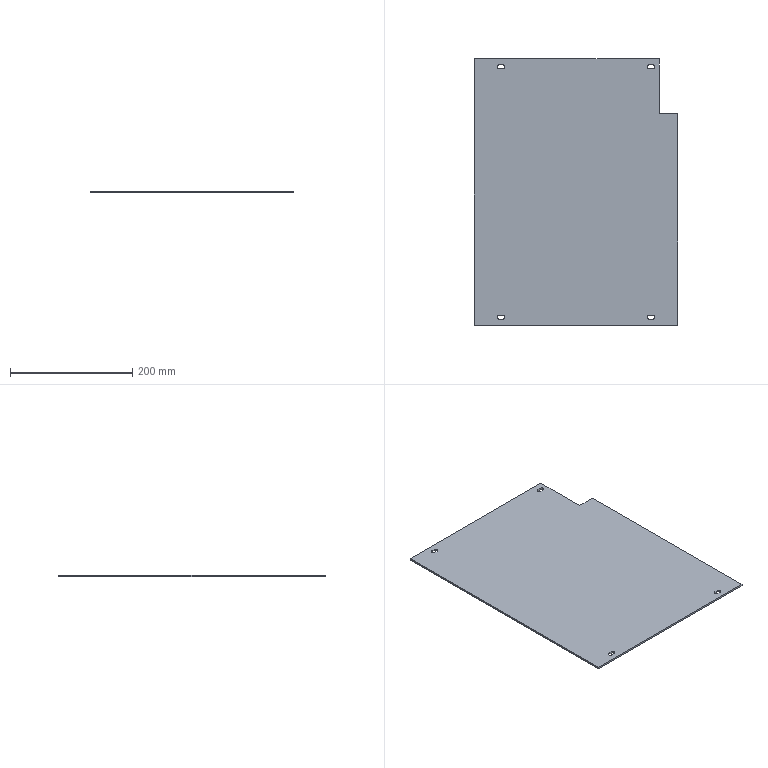Part | SolidWorks | features Cut 2, Extrusion 1 | 1 solid | 28 faces | box 333 x 436 x 3 mm | volume 426578 mm3 | plane 16 | cylinder 12 | commonest cylinder face diameters 6.6 x12
STEP:
#1=CARTESIAN_POINT('',(-116.7,-205.,0.));
#2=VERTEX_POINT('',#1);
#3=CARTESIAN_POINT('',(-120.,-201.7,0.));
#4=VERTEX_POINT('',#3);
#5=CARTESIAN_POINT('',(-120.,-205.,0.));
#6=DIRECTION('',(0.,0.,1.));
#7=DIRECTION('',(1.,0.,0.));
#8=AXIS2_PLACEMENT_3D('',#5,#6,#7);
#9=CIRCLE('',#8,3.3);
#10=EDGE_CURVE('',#2,#4,#9,.T.);
#11=ORIENTED_EDGE('',*,*,#10,.F.);
#12=CARTESIAN_POINT('',(-116.7,-205.,3.));
#13=VERTEX_POINT('',#12);
#14=CARTESIAN_POINT('',(-116.7,-205.,-7.));
#15=DIRECTION('',(0.,0.,1.));
#16=VECTOR('',#15,1000.);
#17=LINE('',#14,#16);
#18=EDGE_CURVE('',#2,#13,#17,.T.);
#19=ORIENTED_EDGE('',*,*,#18,.T.);
#20=CARTESIAN_POINT('',(-120.,-201.7,3.));
#21=VERTEX_POINT('',#20);
#22=CARTESIAN_POINT('',(-120.,-205.,3.));
#23=DIRECTION('',(0.,0.,1.));
#24=DIRECTION('',(1.,0.,0.));
#25=AXIS2_PLACEMENT_3D('',#22,#23,#24);
#26=CIRCLE('',#25,3.3);
#27=EDGE_CURVE('',#13,#21,#26,.T.);
#28=ORIENTED_EDGE('',*,*,#27,.T.);
#29=CARTESIAN_POINT('',(-120.,-201.7,-7.));
#30=DIRECTION('',(0.,0.,1.));
#31=VECTOR('',#30,1000.);
#32=LINE('',#29,#31);
#33=EDGE_CURVE('',#4,#21,#32,.T.);
#34=ORIENTED_EDGE('',*,*,#33,.F.);
#35=EDGE_LOOP('',(#11,#19,#28,#34));
#36=FACE_OUTER_BOUND('',#35,.T.);
#37=CARTESIAN_POINT('',(-120.,-205.,-7.));
#38=DIRECTION('',(0.,0.,1.));
#39=DIRECTION('',(1.,0.,0.));
#40=AXIS2_PLACEMENT_3D('',#37,#38,#39);
#41=CYLINDRICAL_SURFACE('',#40,3.3);
#42=ADVANCED_FACE('',(#36),#41,.F.);
#43=CARTESIAN_POINT('',(129.3,-205.,0.));
#44=VERTEX_POINT('',#43);
#45=CARTESIAN_POINT('',(126.,-201.7,0.));
#46=VERTEX_POINT('',#45);
#47=CARTESIAN_POINT('',(126.,-205.,0.));
#48=DIRECTION('',(0.,0.,1.));
#49=DIRECTION('',(1.,0.,0.));
#50=AXIS2_PLACEMENT_3D('',#47,#48,#49);
#51=CIRCLE('',#50,3.3);
#52=EDGE_CURVE('',#44,#46,#51,.T.);
#53=ORIENTED_EDGE('',*,*,#52,.F.);
#54=CARTESIAN_POINT('',(129.3,-205.,3.));
#55=VERTEX_POINT('',#54);
#56=CARTESIAN_POINT('',(129.3,-205.,-7.));
#57=DIRECTION('',(0.,0.,1.));
#58=VECTOR('',#57,1000.);
#59=LINE('',#56,#58);
#60=EDGE_CURVE('',#44,#55,#59,.T.);
#61=ORIENTED_EDGE('',*,*,#60,.T.);
#62=CARTESIAN_POINT('',(126.,-201.7,3.));
#63=VERTEX_POINT('',#62);
#64=CARTESIAN_POINT('',(126.,-205.,3.));
#65=DIRECTION('',(0.,0.,1.));
#66=DIRECTION('',(1.,0.,0.));
#67=AXIS2_PLACEMENT_3D('',#64,#65,#66);
#68=CIRCLE('',#67,3.3);
#69=EDGE_CURVE('',#55,#63,#68,.T.);
#70=ORIENTED_EDGE('',*,*,#69,.T.);
#71=CARTESIAN_POINT('',(126.,-201.7,-7.));
#72=DIRECTION('',(0.,0.,1.));
#73=VECTOR('',#72,1000.);
#74=LINE('',#71,#73);
#75=EDGE_CURVE('',#46,#63,#74,.T.);
#76=ORIENTED_EDGE('',*,*,#75,.F.);
#77=EDGE_LOOP('',(#53,#61,#70,#76));
#78=FACE_OUTER_BOUND('',#77,.T.);
#79=CARTESIAN_POINT('',(126.,-205.,-7.));
#80=DIRECTION('',(0.,0.,1.));
#81=DIRECTION('',(1.,0.,0.));
#82=AXIS2_PLACEMENT_3D('',#79,#80,#81);
#83=CYLINDRICAL_SURFACE('',#82,3.3);
#84=ADVANCED_FACE('',(#78),#83,.F.);
#85=CARTESIAN_POINT('',(129.3,205.,0.));
#86=VERTEX_POINT('',#85);
#87=CARTESIAN_POINT('',(126.,208.3,0.));
#88=VERTEX_POINT('',#87);
#89=CARTESIAN_POINT('',(126.,205.,0.));
#90=DIRECTION('',(0.,0.,1.));
#91=DIRECTION('',(1.,0.,0.));
#92=AXIS2_PLACEMENT_3D('',#89,#90,#91);
#93=CIRCLE('',#92,3.3);
#94=EDGE_CURVE('',#86,#88,#93,.T.);
#95=ORIENTED_EDGE('',*,*,#94,.F.);
#96=CARTESIAN_POINT('',(129.3,205.,3.));
#97=VERTEX_POINT('',#96);
#98=CARTESIAN_POINT('',(129.3,205.,-7.));
#99=DIRECTION('',(0.,0.,1.));
#100=VECTOR('',#99,1000.);
#101=LINE('',#98,#100);
#102=EDGE_CURVE('',#86,#97,#101,.T.);
#103=ORIENTED_EDGE('',*,*,#102,.T.);
#104=CARTESIAN_POINT('',(126.,208.3,3.));
#105=VERTEX_POINT('',#104);
#106=CARTESIAN_POINT('',(126.,205.,3.));
#107=DIRECTION('',(0.,0.,1.));
#108=DIRECTION('',(1.,0.,0.));
#109=AXIS2_PLACEMENT_3D('',#106,#107,#108);
#110=CIRCLE('',#109,3.3);
#111=EDGE_CURVE('',#97,#105,#110,.T.);
#112=ORIENTED_EDGE('',*,*,#111,.T.);
#113=CARTESIAN_POINT('',(126.,208.3,-7.));
#114=DIRECTION('',(0.,0.,1.));
#115=VECTOR('',#114,1000.);
#116=LINE('',#113,#115);
#117=EDGE_CURVE('',#88,#105,#116,.T.);
#118=ORIENTED_EDGE('',*,*,#117,.F.);
#119=EDGE_LOOP('',(#95,#103,#112,#118));
#120=FACE_OUTER_BOUND('',#119,.T.);
#121=CARTESIAN_POINT('',(126.,205.,-7.));
#122=DIRECTION('',(0.,0.,1.));
#123=DIRECTION('',(1.,0.,0.));
#124=AXIS2_PLACEMENT_3D('',#121,#122,#123);
#125=CYLINDRICAL_SURFACE('',#124,3.3);
#126=ADVANCED_FACE('',(#120),#125,.F.);
#127=CARTESIAN_POINT('',(-116.7,205.,0.));
#128=VERTEX_POINT('',#127);
#129=CARTESIAN_POINT('',(-120.,208.3,0.));
#130=VERTEX_POINT('',#129);
#131=CARTESIAN_POINT('',(-120.,205.,0.));
#132=DIRECTION('',(0.,0.,1.));
#133=DIRECTION('',(1.,0.,0.));
#134=AXIS2_PLACEMENT_3D('',#131,#132,#133);
#135=CIRCLE('',#134,3.3);
#136=EDGE_CURVE('',#128,#130,#135,.T.);
#137=ORIENTED_EDGE('',*,*,#136,.F.);
#138=CARTESIAN_POINT('',(-116.7,205.,3.));
#139=VERTEX_POINT('',#138);
#140=CARTESIAN_POINT('',(-116.7,205.,-7.));
#141=DIRECTION('',(0.,0.,1.));
#142=VECTOR('',#141,1000.);
#143=LINE('',#140,#142);
#144=EDGE_CURVE('',#128,#139,#143,.T.);
#145=ORIENTED_EDGE('',*,*,#144,.T.);
#146=CARTESIAN_POINT('',(-120.,208.3,3.));
#147=VERTEX_POINT('',#146);
#148=CARTESIAN_POINT('',(-120.,205.,3.));
#149=DIRECTION('',(0.,0.,1.));
#150=DIRECTION('',(1.,0.,0.));
#151=AXIS2_PLACEMENT_3D('',#148,#149,#150);
#152=CIRCLE('',#151,3.3);
#153=EDGE_CURVE('',#139,#147,#152,.T.);
#154=ORIENTED_EDGE('',*,*,#153,.T.);
#155=CARTESIAN_POINT('',(-120.,208.3,-7.));
#156=DIRECTION('',(0.,0.,1.));
#157=VECTOR('',#156,1000.);
#158=LINE('',#155,#157);
#159=EDGE_CURVE('',#130,#147,#158,.T.);
#160=ORIENTED_EDGE('',*,*,#159,.F.);
#161=EDGE_LOOP('',(#137,#145,#154,#160));
#162=FACE_OUTER_BOUND('',#161,.T.);
#163=CARTESIAN_POINT('',(-120.,205.,-7.));
#164=DIRECTION('',(0.,0.,1.));
#165=DIRECTION('',(1.,0.,0.));
#166=AXIS2_PLACEMENT_3D('',#163,#164,#165);
#167=CYLINDRICAL_SURFACE('',#166,3.3);
#168=ADVANCED_FACE('',(#162),#167,.F.);
#169=CARTESIAN_POINT('',(-166.5,218.,0.));
#170=VERTEX_POINT('',#169);
#171=CARTESIAN_POINT('',(-166.5,-218.,0.));
#172=VERTEX_POINT('',#171);
#173=CARTESIAN_POINT('',(-166.5,-218.,0.));
#174=DIRECTION('',(0.,-1.,0.));
#175=VECTOR('',#174,1000.);
#176=LINE('',#173,#175);
#177=EDGE_CURVE('',#170,#172,#176,.T.);
#178=ORIENTED_EDGE('',*,*,#177,.T.);
#179=CARTESIAN_POINT('',(-166.5,-218.,3.));
#180=VERTEX_POINT('',#179);
#181=CARTESIAN_POINT('',(-166.5,-218.,3.));
#182=DIRECTION('',(0.,0.,-1.));
#183=VECTOR('',#182,1000.);
#184=LINE('',#181,#183);
#185=EDGE_CURVE('',#180,#172,#184,.T.);
#186=ORIENTED_EDGE('',*,*,#185,.F.);
#187=CARTESIAN_POINT('',(-166.5,218.,3.));
#188=VERTEX_POINT('',#187);
#189=CARTESIAN_POINT('',(-166.5,-218.,3.));
#190=DIRECTION('',(0.,-1.,0.));
#191=VECTOR('',#190,1000.);
#192=LINE('',#189,#191);
#193=EDGE_CURVE('',#188,#180,#192,.T.);
#194=ORIENTED_EDGE('',*,*,#193,.F.);
#195=CARTESIAN_POINT('',(-166.5,218.,3.));
#196=DIRECTION('',(0.,0.,-1.));
#197=VECTOR('',#196,1000.);
#198=LINE('',#195,#197);
#199=EDGE_CURVE('',#188,#170,#198,.T.);
#200=ORIENTED_EDGE('',*,*,#199,.T.);
#201=EDGE_LOOP('',(#178,#186,#194,#200));
#202=FACE_OUTER_BOUND('',#201,.T.);
#203=CARTESIAN_POINT('',(-166.5,-218.,3.));
#204=DIRECTION('',(1.,0.,0.));
#205=DIRECTION('',(0.,0.,-1.));
#206=AXIS2_PLACEMENT_3D('',#203,#204,#205);
#207=PLANE('',#206);
#208=ADVANCED_FACE('',(#202),#207,.F.);
#209=CARTESIAN_POINT('',(166.5,-218.,0.));
#210=VERTEX_POINT('',#209);
#211=CARTESIAN_POINT('',(166.5,-218.,0.));
#212=DIRECTION('',(1.,0.,0.));
#213=VECTOR('',#212,1000.);
#214=LINE('',#211,#213);
#215=EDGE_CURVE('',#172,#210,#214,.T.);
#216=ORIENTED_EDGE('',*,*,#215,.T.);
#217=CARTESIAN_POINT('',(166.5,-218.,3.));
#218=VERTEX_POINT('',#217);
#219=CARTESIAN_POINT('',(166.5,-218.,3.));
#220=DIRECTION('',(0.,0.,-1.));
#221=VECTOR('',#220,1000.);
#222=LINE('',#219,#221);
#223=EDGE_CURVE('',#218,#210,#222,.T.);
#224=ORIENTED_EDGE('',*,*,#223,.F.);
#225=CARTESIAN_POINT('',(166.5,-218.,3.));
#226=DIRECTION('',(1.,0.,0.));
#227=VECTOR('',#226,1000.);
#228=LINE('',#225,#227);
#229=EDGE_CURVE('',#180,#218,#228,.T.);
#230=ORIENTED_EDGE('',*,*,#229,.F.);
#231=ORIENTED_EDGE('',*,*,#185,.T.);
#232=EDGE_LOOP('',(#216,#224,#230,#231));
#233=FACE_OUTER_BOUND('',#232,.T.);
#234=CARTESIAN_POINT('',(166.5,-218.,3.));
#235=DIRECTION('',(0.,1.,0.));
#236=DIRECTION('',(-1.,0.,0.));
#237=AXIS2_PLACEMENT_3D('',#234,#235,#236);
#238=PLANE('',#237);
#239=ADVANCED_FACE('',(#233),#238,.F.);
#240=CARTESIAN_POINT('',(166.5,128.,0.));
#241=VERTEX_POINT('',#240);
#242=CARTESIAN_POINT('',(166.5,-218.,0.));
#243=DIRECTION('',(0.,1.,0.));
#244=VECTOR('',#243,1000.);
#245=LINE('',#242,#244);
#246=EDGE_CURVE('',#210,#241,#245,.T.);
#247=ORIENTED_EDGE('',*,*,#246,.T.);
#248=CARTESIAN_POINT('',(166.5,128.,3.));
#249=VERTEX_POINT('',#248);
#250=CARTESIAN_POINT('',(166.5,128.,10.));
#251=DIRECTION('',(0.,0.,-1.));
#252=VECTOR('',#251,1000.);
#253=LINE('',#250,#252);
#254=EDGE_CURVE('',#249,#241,#253,.T.);
#255=ORIENTED_EDGE('',*,*,#254,.F.);
#256=CARTESIAN_POINT('',(166.5,-218.,3.));
#257=DIRECTION('',(0.,1.,0.));
#258=VECTOR('',#257,1000.);
#259=LINE('',#256,#258);
#260=EDGE_CURVE('',#218,#249,#259,.T.);
#261=ORIENTED_EDGE('',*,*,#260,.F.);
#262=ORIENTED_EDGE('',*,*,#223,.T.);
#263=EDGE_LOOP('',(#247,#255,#261,#262));
#264=FACE_OUTER_BOUND('',#263,.T.);
#265=CARTESIAN_POINT('',(166.5,-218.,3.));
#266=DIRECTION('',(-1.,0.,0.));
#267=DIRECTION('',(0.,0.,1.));
#268=AXIS2_PLACEMENT_3D('',#265,#266,#267);
#269=PLANE('',#268);
#270=ADVANCED_FACE('',(#264),#269,.F.);
#271=CARTESIAN_POINT('',(136.5,218.,3.));
#272=VERTEX_POINT('',#271);
#273=CARTESIAN_POINT('',(166.5,218.,3.));
#274=DIRECTION('',(-1.,0.,0.));
#275=VECTOR('',#274,1000.);
#276=LINE('',#273,#275);
#277=EDGE_CURVE('',#272,#188,#276,.T.);
#278=ORIENTED_EDGE('',*,*,#277,.F.);
#279=CARTESIAN_POINT('',(136.5,218.,0.));
#280=VERTEX_POINT('',#279);
#281=CARTESIAN_POINT('',(136.5,218.,10.));
#282=DIRECTION('',(0.,0.,-1.));
#283=VECTOR('',#282,1000.);
#284=LINE('',#281,#283);
#285=EDGE_CURVE('',#272,#280,#284,.T.);
#286=ORIENTED_EDGE('',*,*,#285,.T.);
#287=CARTESIAN_POINT('',(166.5,218.,0.));
#288=DIRECTION('',(-1.,0.,0.));
#289=VECTOR('',#288,1000.);
#290=LINE('',#287,#289);
#291=EDGE_CURVE('',#280,#170,#290,.T.);
#292=ORIENTED_EDGE('',*,*,#291,.T.);
#293=ORIENTED_EDGE('',*,*,#199,.F.);
#294=EDGE_LOOP('',(#278,#286,#292,#293));
#295=FACE_OUTER_BOUND('',#294,.T.);
#296=CARTESIAN_POINT('',(166.5,218.,3.));
#297=DIRECTION('',(0.,-1.,0.));
#298=DIRECTION('',(1.,0.,0.));
#299=AXIS2_PLACEMENT_3D('',#296,#297,#298);
#300=PLANE('',#299);
#301=ADVANCED_FACE('',(#295),#300,.F.);
#302=CARTESIAN_POINT('',(-120.,-208.3,3.));
#303=VERTEX_POINT('',#302);
#304=CARTESIAN_POINT('',(-120.,-205.,3.));
#305=DIRECTION('',(0.,0.,1.));
#306=DIRECTION('',(1.,0.,0.));
#307=AXIS2_PLACEMENT_3D('',#304,#305,#306);
#308=CIRCLE('',#307,3.3);
#309=EDGE_CURVE('',#303,#13,#308,.T.);
#310=ORIENTED_EDGE('',*,*,#309,.F.);
#311=CARTESIAN_POINT('',(-126.,-208.3,3.));
#312=VERTEX_POINT('',#311);
#313=CARTESIAN_POINT('',(-120.,-208.3,3.));
#314=DIRECTION('',(1.,0.,0.));
#315=VECTOR('',#314,1000.);
#316=LINE('',#313,#315);
#317=EDGE_CURVE('',#312,#303,#316,.T.);
#318=ORIENTED_EDGE('',*,*,#317,.F.);
#319=CARTESIAN_POINT('',(-126.,-201.7,3.));
#320=VERTEX_POINT('',#319);
#321=CARTESIAN_POINT('',(-126.,-205.,3.));
#322=DIRECTION('',(0.,0.,1.));
#323=DIRECTION('',(1.,0.,0.));
#324=AXIS2_PLACEMENT_3D('',#321,#322,#323);
#325=CIRCLE('',#324,3.3);
#326=EDGE_CURVE('',#320,#312,#325,.T.);
#327=ORIENTED_EDGE('',*,*,#326,.F.);
#328=CARTESIAN_POINT('',(-120.,-201.7,3.));
#329=DIRECTION('',(-1.,0.,0.));
#330=VECTOR('',#329,1000.);
#331=LINE('',#328,#330);
#332=EDGE_CURVE('',#21,#320,#331,.T.);
#333=ORIENTED_EDGE('',*,*,#332,.F.);
#334=ORIENTED_EDGE('',*,*,#27,.F.);
#335=EDGE_LOOP('',(#310,#318,#327,#333,#334));
#336=FACE_BOUND('',#335,.T.);
#337=CARTESIAN_POINT('',(120.,-201.7,3.));
#338=VERTEX_POINT('',#337);
#339=CARTESIAN_POINT('',(120.,-208.3,3.));
#340=VERTEX_POINT('',#339);
#341=CARTESIAN_POINT('',(120.,-205.,3.));
#342=DIRECTION('',(0.,0.,1.));
#343=DIRECTION('',(1.,0.,0.));
#344=AXIS2_PLACEMENT_3D('',#341,#342,#343);
#345=CIRCLE('',#344,3.3);
#346=EDGE_CURVE('',#338,#340,#345,.T.);
#347=ORIENTED_EDGE('',*,*,#346,.F.);
#348=CARTESIAN_POINT('',(120.,-201.7,3.));
#349=DIRECTION('',(-1.,0.,0.));
#350=VECTOR('',#349,1000.);
#351=LINE('',#348,#350);
#352=EDGE_CURVE('',#63,#338,#351,.T.);
#353=ORIENTED_EDGE('',*,*,#352,.F.);
#354=ORIENTED_EDGE('',*,*,#69,.F.);
#355=CARTESIAN_POINT('',(126.,-208.3,3.));
#356=VERTEX_POINT('',#355);
#357=CARTESIAN_POINT('',(126.,-205.,3.));
#358=DIRECTION('',(0.,0.,1.));
#359=DIRECTION('',(1.,0.,0.));
#360=AXIS2_PLACEMENT_3D('',#357,#358,#359);
#361=CIRCLE('',#360,3.3);
#362=EDGE_CURVE('',#356,#55,#361,.T.);
#363=ORIENTED_EDGE('',*,*,#362,.F.);
#364=CARTESIAN_POINT('',(120.,-208.3,3.));
#365=DIRECTION('',(1.,0.,0.));
#366=VECTOR('',#365,1000.);
#367=LINE('',#364,#366);
#368=EDGE_CURVE('',#340,#356,#367,.T.);
#369=ORIENTED_EDGE('',*,*,#368,.F.);
#370=EDGE_LOOP('',(#347,#353,#354,#363,#369));
#371=FACE_BOUND('',#370,.T.);
#372=CARTESIAN_POINT('',(120.,208.3,3.));
#373=VERTEX_POINT('',#372);
#374=CARTESIAN_POINT('',(120.,201.7,3.));
#375=VERTEX_POINT('',#374);
#376=CARTESIAN_POINT('',(120.,205.,3.));
#377=DIRECTION('',(0.,0.,1.));
#378=DIRECTION('',(1.,0.,0.));
#379=AXIS2_PLACEMENT_3D('',#376,#377,#378);
#380=CIRCLE('',#379,3.3);
#381=EDGE_CURVE('',#373,#375,#380,.T.);
#382=ORIENTED_EDGE('',*,*,#381,.F.);
#383=CARTESIAN_POINT('',(120.,208.3,3.));
#384=DIRECTION('',(-1.,0.,0.));
#385=VECTOR('',#384,1000.);
#386=LINE('',#383,#385);
#387=EDGE_CURVE('',#105,#373,#386,.T.);
#388=ORIENTED_EDGE('',*,*,#387,.F.);
#389=ORIENTED_EDGE('',*,*,#111,.F.);
#390=CARTESIAN_POINT('',(126.,201.7,3.));
#391=VERTEX_POINT('',#390);
#392=CARTESIAN_POINT('',(126.,205.,3.));
#393=DIRECTION('',(0.,0.,1.));
#394=DIRECTION('',(1.,0.,0.));
#395=AXIS2_PLACEMENT_3D('',#392,#393,#394);
#396=CIRCLE('',#395,3.3);
#397=EDGE_CURVE('',#391,#97,#396,.T.);
#398=ORIENTED_EDGE('',*,*,#397,.F.);
#399=CARTESIAN_POINT('',(120.,201.7,3.));
#400=DIRECTION('',(1.,0.,0.));
#401=VECTOR('',#400,1000.);
#402=LINE('',#399,#401);
#403=EDGE_CURVE('',#375,#391,#402,.T.);
#404=ORIENTED_EDGE('',*,*,#403,.F.);
#405=EDGE_LOOP('',(#382,#388,#389,#398,#404));
#406=FACE_BOUND('',#405,.T.);
#407=CARTESIAN_POINT('',(-120.,201.7,3.));
#408=VERTEX_POINT('',#407);
#409=CARTESIAN_POINT('',(-120.,205.,3.));
#410=DIRECTION('',(0.,0.,1.));
#411=DIRECTION('',(1.,0.,0.));
#412=AXIS2_PLACEMENT_3D('',#409,#410,#411);
#413=CIRCLE('',#412,3.3);
#414=EDGE_CURVE('',#408,#139,#413,.T.);
#415=ORIENTED_EDGE('',*,*,#414,.F.);
#416=CARTESIAN_POINT('',(-126.,201.7,3.));
#417=VERTEX_POINT('',#416);
#418=CARTESIAN_POINT('',(-120.,201.7,3.));
#419=DIRECTION('',(1.,0.,0.));
#420=VECTOR('',#419,1000.);
#421=LINE('',#418,#420);
#422=EDGE_CURVE('',#417,#408,#421,.T.);
#423=ORIENTED_EDGE('',*,*,#422,.F.);
#424=CARTESIAN_POINT('',(-126.,208.3,3.));
#425=VERTEX_POINT('',#424);
#426=CARTESIAN_POINT('',(-126.,205.,3.));
#427=DIRECTION('',(0.,0.,1.));
#428=DIRECTION('',(1.,0.,0.));
#429=AXIS2_PLACEMENT_3D('',#426,#427,#428);
#430=CIRCLE('',#429,3.3);
#431=EDGE_CURVE('',#425,#417,#430,.T.);
#432=ORIENTED_EDGE('',*,*,#431,.F.);
#433=CARTESIAN_POINT('',(-120.,208.3,3.));
#434=DIRECTION('',(-1.,0.,0.));
#435=VECTOR('',#434,1000.);
#436=LINE('',#433,#435);
#437=EDGE_CURVE('',#147,#425,#436,.T.);
#438=ORIENTED_EDGE('',*,*,#437,.F.);
#439=ORIENTED_EDGE('',*,*,#153,.F.);
#440=EDGE_LOOP('',(#415,#423,#432,#438,#439));
#441=FACE_BOUND('',#440,.T.);
#442=CARTESIAN_POINT('',(136.5,128.,3.));
#443=VERTEX_POINT('',#442);
#444=CARTESIAN_POINT('',(136.5,0.,3.));
#445=DIRECTION('',(0.,-1.,0.));
#446=VECTOR('',#445,1000.);
#447=LINE('',#444,#446);
#448=EDGE_CURVE('',#272,#443,#447,.T.);
#449=ORIENTED_EDGE('',*,*,#448,.F.);
#450=ORIENTED_EDGE('',*,*,#277,.T.);
#451=ORIENTED_EDGE('',*,*,#193,.T.);
#452=ORIENTED_EDGE('',*,*,#229,.T.);
#453=ORIENTED_EDGE('',*,*,#260,.T.);
#454=CARTESIAN_POINT('',(0.,128.,3.));
#455=DIRECTION('',(1.,0.,0.));
#456=VECTOR('',#455,1000.);
#457=LINE('',#454,#456);
#458=EDGE_CURVE('',#443,#249,#457,.T.);
#459=ORIENTED_EDGE('',*,*,#458,.F.);
#460=EDGE_LOOP('',(#449,#450,#451,#452,#453,#459));
#461=FACE_OUTER_BOUND('',#460,.T.);
#462=CARTESIAN_POINT('',(0.,0.,3.));
#463=DIRECTION('',(0.,0.,1.));
#464=DIRECTION('',(1.,0.,0.));
#465=AXIS2_PLACEMENT_3D('',#462,#463,#464);
#466=PLANE('',#465);
#467=ADVANCED_FACE('',(#336,#371,#406,#441,#461),#466,.T.);
#468=CARTESIAN_POINT('',(-126.,-208.3,0.));
#469=VERTEX_POINT('',#468);
#470=CARTESIAN_POINT('',(-120.,-208.3,0.));
#471=VERTEX_POINT('',#470);
#472=CARTESIAN_POINT('',(0.,-208.3,0.));
#473=DIRECTION('',(1.,0.,0.));
#474=VECTOR('',#473,1000.);
#475=LINE('',#472,#474);
#476=EDGE_CURVE('',#469,#471,#475,.T.);
#477=ORIENTED_EDGE('',*,*,#476,.T.);
#478=CARTESIAN_POINT('',(-120.,-205.,0.));
#479=DIRECTION('',(0.,0.,1.));
#480=DIRECTION('',(1.,0.,0.));
#481=AXIS2_PLACEMENT_3D('',#478,#479,#480);
#482=CIRCLE('',#481,3.3);
#483=EDGE_CURVE('',#471,#2,#482,.T.);
#484=ORIENTED_EDGE('',*,*,#483,.T.);
#485=ORIENTED_EDGE('',*,*,#10,.T.);
#486=CARTESIAN_POINT('',(-126.,-201.7,0.));
#487=VERTEX_POINT('',#486);
#488=CARTESIAN_POINT('',(0.,-201.7,0.));
#489=DIRECTION('',(-1.,0.,0.));
#490=VECTOR('',#489,1000.);
#491=LINE('',#488,#490);
#492=EDGE_CURVE('',#4,#487,#491,.T.);
#493=ORIENTED_EDGE('',*,*,#492,.T.);
#494=CARTESIAN_POINT('',(-126.,-205.,0.));
#495=DIRECTION('',(0.,0.,1.));
#496=DIRECTION('',(1.,0.,0.));
#497=AXIS2_PLACEMENT_3D('',#494,#495,#496);
#498=CIRCLE('',#497,3.3);
#499=EDGE_CURVE('',#487,#469,#498,.T.);
#500=ORIENTED_EDGE('',*,*,#499,.T.);
#501=EDGE_LOOP('',(#477,#484,#485,#493,#500));
#502=FACE_BOUND('',#501,.T.);
#503=CARTESIAN_POINT('',(120.,-201.7,0.));
#504=VERTEX_POINT('',#503);
#505=CARTESIAN_POINT('',(0.,-201.7,0.));
#506=DIRECTION('',(-1.,0.,0.));
#507=VECTOR('',#506,1000.);
#508=LINE('',#505,#507);
#509=EDGE_CURVE('',#46,#504,#508,.T.);
#510=ORIENTED_EDGE('',*,*,#509,.T.);
#511=CARTESIAN_POINT('',(120.,-208.3,0.));
#512=VERTEX_POINT('',#511);
#513=CARTESIAN_POINT('',(120.,-205.,0.));
#514=DIRECTION('',(0.,0.,1.));
#515=DIRECTION('',(1.,0.,0.));
#516=AXIS2_PLACEMENT_3D('',#513,#514,#515);
#517=CIRCLE('',#516,3.3);
#518=EDGE_CURVE('',#504,#512,#517,.T.);
#519=ORIENTED_EDGE('',*,*,#518,.T.);
#520=CARTESIAN_POINT('',(126.,-208.3,0.));
#521=VERTEX_POINT('',#520);
#522=CARTESIAN_POINT('',(0.,-208.3,0.));
#523=DIRECTION('',(1.,0.,0.));
#524=VECTOR('',#523,1000.);
#525=LINE('',#522,#524);
#526=EDGE_CURVE('',#512,#521,#525,.T.);
#527=ORIENTED_EDGE('',*,*,#526,.T.);
#528=CARTESIAN_POINT('',(126.,-205.,0.));
#529=DIRECTION('',(0.,0.,1.));
#530=DIRECTION('',(1.,0.,0.));
#531=AXIS2_PLACEMENT_3D('',#528,#529,#530);
#532=CIRCLE('',#531,3.3);
#533=EDGE_CURVE('',#521,#44,#532,.T.);
#534=ORIENTED_EDGE('',*,*,#533,.T.);
#535=ORIENTED_EDGE('',*,*,#52,.T.);
#536=EDGE_LOOP('',(#510,#519,#527,#534,#535));
#537=FACE_BOUND('',#536,.T.);
#538=CARTESIAN_POINT('',(120.,208.3,0.));
#539=VERTEX_POINT('',#538);
#540=CARTESIAN_POINT('',(0.,208.3,0.));
#541=DIRECTION('',(-1.,0.,0.));
#542=VECTOR('',#541,1000.);
#543=LINE('',#540,#542);
#544=EDGE_CURVE('',#88,#539,#543,.T.);
#545=ORIENTED_EDGE('',*,*,#544,.T.);
#546=CARTESIAN_POINT('',(120.,201.7,0.));
#547=VERTEX_POINT('',#546);
#548=CARTESIAN_POINT('',(120.,205.,0.));
#549=DIRECTION('',(0.,0.,1.));
#550=DIRECTION('',(1.,0.,0.));
#551=AXIS2_PLACEMENT_3D('',#548,#549,#550);
#552=CIRCLE('',#551,3.3);
#553=EDGE_CURVE('',#539,#547,#552,.T.);
#554=ORIENTED_EDGE('',*,*,#553,.T.);
#555=CARTESIAN_POINT('',(126.,201.7,0.));
#556=VERTEX_POINT('',#555);
#557=CARTESIAN_POINT('',(0.,201.7,0.));
#558=DIRECTION('',(1.,0.,0.));
#559=VECTOR('',#558,1000.);
#560=LINE('',#557,#559);
#561=EDGE_CURVE('',#547,#556,#560,.T.);
#562=ORIENTED_EDGE('',*,*,#561,.T.);
#563=CARTESIAN_POINT('',(126.,205.,0.));
#564=DIRECTION('',(0.,0.,1.));
#565=DIRECTION('',(1.,0.,0.));
#566=AXIS2_PLACEMENT_3D('',#563,#564,#565);
#567=CIRCLE('',#566,3.3);
#568=EDGE_CURVE('',#556,#86,#567,.T.);
#569=ORIENTED_EDGE('',*,*,#568,.T.);
#570=ORIENTED_EDGE('',*,*,#94,.T.);
#571=EDGE_LOOP('',(#545,#554,#562,#569,#570));
#572=FACE_BOUND('',#571,.T.);
#573=CARTESIAN_POINT('',(-126.,201.7,0.));
#574=VERTEX_POINT('',#573);
#575=CARTESIAN_POINT('',(-120.,201.7,0.));
#576=VERTEX_POINT('',#575);
#577=CARTESIAN_POINT('',(0.,201.7,0.));
#578=DIRECTION('',(1.,0.,0.));
#579=VECTOR('',#578,1000.);
#580=LINE('',#577,#579);
#581=EDGE_CURVE('',#574,#576,#580,.T.);
#582=ORIENTED_EDGE('',*,*,#581,.T.);
#583=CARTESIAN_POINT('',(-120.,205.,0.));
#584=DIRECTION('',(0.,0.,1.));
#585=DIRECTION('',(1.,0.,0.));
#586=AXIS2_PLACEMENT_3D('',#583,#584,#585);
#587=CIRCLE('',#586,3.3);
#588=EDGE_CURVE('',#576,#128,#587,.T.);
#589=ORIENTED_EDGE('',*,*,#588,.T.);
#590=ORIENTED_EDGE('',*,*,#136,.T.);
#591=CARTESIAN_POINT('',(-126.,208.3,0.));
#592=VERTEX_POINT('',#591);
#593=CARTESIAN_POINT('',(0.,208.3,0.));
#594=DIRECTION('',(-1.,0.,0.));
#595=VECTOR('',#594,1000.);
#596=LINE('',#593,#595);
#597=EDGE_CURVE('',#130,#592,#596,.T.);
#598=ORIENTED_EDGE('',*,*,#597,.T.);
#599=CARTESIAN_POINT('',(-126.,205.,0.));
#600=DIRECTION('',(0.,0.,1.));
#601=DIRECTION('',(1.,0.,0.));
#602=AXIS2_PLACEMENT_3D('',#599,#600,#601);
#603=CIRCLE('',#602,3.3);
#604=EDGE_CURVE('',#592,#574,#603,.T.);
#605=ORIENTED_EDGE('',*,*,#604,.T.);
#606=EDGE_LOOP('',(#582,#589,#590,#598,#605));
#607=FACE_BOUND('',#606,.T.);
#608=ORIENTED_EDGE('',*,*,#291,.F.);
#609=CARTESIAN_POINT('',(136.5,128.,0.));
#610=VERTEX_POINT('',#609);
#611=CARTESIAN_POINT('',(136.5,128.,0.));
#612=DIRECTION('',(0.,1.,0.));
#613=VECTOR('',#612,1000.);
#614=LINE('',#611,#613);
#615=EDGE_CURVE('',#610,#280,#614,.T.);
#616=ORIENTED_EDGE('',*,*,#615,.F.);
#617=CARTESIAN_POINT('',(136.5,128.,0.));
#618=DIRECTION('',(-1.,0.,0.));
#619=VECTOR('',#618,1000.);
#620=LINE('',#617,#619);
#621=EDGE_CURVE('',#241,#610,#620,.T.);
#622=ORIENTED_EDGE('',*,*,#621,.F.);
#623=ORIENTED_EDGE('',*,*,#246,.F.);
#624=ORIENTED_EDGE('',*,*,#215,.F.);
#625=ORIENTED_EDGE('',*,*,#177,.F.);
#626=EDGE_LOOP('',(#608,#616,#622,#623,#624,#625));
#627=FACE_OUTER_BOUND('',#626,.T.);
#628=CARTESIAN_POINT('',(0.,0.,0.));
#629=DIRECTION('',(0.,0.,1.));
#630=DIRECTION('',(1.,0.,0.));
#631=AXIS2_PLACEMENT_3D('',#628,#629,#630);
#632=PLANE('',#631);
#633=ADVANCED_FACE('',(#502,#537,#572,#607,#627),#632,.F.);
#634=ORIENTED_EDGE('',*,*,#448,.T.);
#635=CARTESIAN_POINT('',(136.5,128.,10.));
#636=DIRECTION('',(0.,0.,-1.));
#637=VECTOR('',#636,1000.);
#638=LINE('',#635,#637);
#639=EDGE_CURVE('',#443,#610,#638,.T.);
#640=ORIENTED_EDGE('',*,*,#639,.T.);
#641=ORIENTED_EDGE('',*,*,#615,.T.);
#642=ORIENTED_EDGE('',*,*,#285,.F.);
#643=EDGE_LOOP('',(#634,#640,#641,#642));
#644=FACE_OUTER_BOUND('',#643,.T.);
#645=CARTESIAN_POINT('',(136.5,128.,10.));
#646=DIRECTION('',(-1.,0.,0.));
#647=DIRECTION('',(0.,0.,1.));
#648=AXIS2_PLACEMENT_3D('',#645,#646,#647);
#649=PLANE('',#648);
#650=ADVANCED_FACE('',(#644),#649,.F.);
#651=ORIENTED_EDGE('',*,*,#458,.T.);
#652=ORIENTED_EDGE('',*,*,#254,.T.);
#653=ORIENTED_EDGE('',*,*,#621,.T.);
#654=ORIENTED_EDGE('',*,*,#639,.F.);
#655=EDGE_LOOP('',(#651,#652,#653,#654));
#656=FACE_OUTER_BOUND('',#655,.T.);
#657=CARTESIAN_POINT('',(136.5,128.,10.));
#658=DIRECTION('',(0.,-1.,0.));
#659=DIRECTION('',(1.,0.,0.));
#660=AXIS2_PLACEMENT_3D('',#657,#658,#659);
#661=PLANE('',#660);
#662=ADVANCED_FACE('',(#656),#661,.F.);
#663=ORIENTED_EDGE('',*,*,#144,.F.);
#664=ORIENTED_EDGE('',*,*,#588,.F.);
#665=CARTESIAN_POINT('',(-120.,201.7,-7.));
#666=DIRECTION('',(0.,0.,1.));
#667=VECTOR('',#666,1000.);
#668=LINE('',#665,#667);
#669=EDGE_CURVE('',#576,#408,#668,.T.);
#670=ORIENTED_EDGE('',*,*,#669,.T.);
#671=ORIENTED_EDGE('',*,*,#414,.T.);
#672=EDGE_LOOP('',(#663,#664,#670,#671));
#673=FACE_OUTER_BOUND('',#672,.T.);
#674=CARTESIAN_POINT('',(-120.,205.,-7.));
#675=DIRECTION('',(0.,0.,1.));
#676=DIRECTION('',(1.,0.,0.));
#677=AXIS2_PLACEMENT_3D('',#674,#675,#676);
#678=CYLINDRICAL_SURFACE('',#677,3.3);
#679=ADVANCED_FACE('',(#673),#678,.F.);
#680=CARTESIAN_POINT('',(-126.,201.7,-7.));
#681=DIRECTION('',(0.,0.,1.));
#682=VECTOR('',#681,1000.);
#683=LINE('',#680,#682);
#684=EDGE_CURVE('',#574,#417,#683,.T.);
#685=ORIENTED_EDGE('',*,*,#684,.T.);
#686=ORIENTED_EDGE('',*,*,#422,.T.);
#687=ORIENTED_EDGE('',*,*,#669,.F.);
#688=ORIENTED_EDGE('',*,*,#581,.F.);
#689=EDGE_LOOP('',(#685,#686,#687,#688));
#690=FACE_OUTER_BOUND('',#689,.T.);
#691=CARTESIAN_POINT('',(-120.,201.7,-7.));
#692=DIRECTION('',(0.,-1.,0.));
#693=DIRECTION('',(1.,0.,0.));
#694=AXIS2_PLACEMENT_3D('',#691,#692,#693);
#695=PLANE('',#694);
#696=ADVANCED_FACE('',(#690),#695,.F.);
#697=CARTESIAN_POINT('',(-126.,208.3,-7.));
#698=DIRECTION('',(0.,0.,1.));
#699=VECTOR('',#698,1000.);
#700=LINE('',#697,#699);
#701=EDGE_CURVE('',#592,#425,#700,.T.);
#702=ORIENTED_EDGE('',*,*,#701,.T.);
#703=ORIENTED_EDGE('',*,*,#431,.T.);
#704=ORIENTED_EDGE('',*,*,#684,.F.);
#705=ORIENTED_EDGE('',*,*,#604,.F.);
#706=EDGE_LOOP('',(#702,#703,#704,#705));
#707=FACE_OUTER_BOUND('',#706,.T.);
#708=CARTESIAN_POINT('',(-126.,205.,-7.));
#709=DIRECTION('',(0.,0.,1.));
#710=DIRECTION('',(1.,0.,0.));
#711=AXIS2_PLACEMENT_3D('',#708,#709,#710);
#712=CYLINDRICAL_SURFACE('',#711,3.3);
#713=ADVANCED_FACE('',(#707),#712,.F.);
#714=ORIENTED_EDGE('',*,*,#159,.T.);
#715=ORIENTED_EDGE('',*,*,#437,.T.);
#716=ORIENTED_EDGE('',*,*,#701,.F.);
#717=ORIENTED_EDGE('',*,*,#597,.F.);
#718=EDGE_LOOP('',(#714,#715,#716,#717));
#719=FACE_OUTER_BOUND('',#718,.T.);
#720=CARTESIAN_POINT('',(-120.,208.3,-7.));
#721=DIRECTION('',(0.,1.,0.));
#722=DIRECTION('',(-1.,0.,0.));
#723=AXIS2_PLACEMENT_3D('',#720,#721,#722);
#724=PLANE('',#723);
#725=ADVANCED_FACE('',(#719),#724,.F.);
#726=CARTESIAN_POINT('',(120.,208.3,-7.));
#727=DIRECTION('',(0.,0.,1.));
#728=VECTOR('',#727,1000.);
#729=LINE('',#726,#728);
#730=EDGE_CURVE('',#539,#373,#729,.T.);
#731=ORIENTED_EDGE('',*,*,#730,.T.);
#732=ORIENTED_EDGE('',*,*,#381,.T.);
#733=CARTESIAN_POINT('',(120.,201.7,-7.));
#734=DIRECTION('',(0.,0.,1.));
#735=VECTOR('',#734,1000.);
#736=LINE('',#733,#735);
#737=EDGE_CURVE('',#547,#375,#736,.T.);
#738=ORIENTED_EDGE('',*,*,#737,.F.);
#739=ORIENTED_EDGE('',*,*,#553,.F.);
#740=EDGE_LOOP('',(#731,#732,#738,#739));
#741=FACE_OUTER_BOUND('',#740,.T.);
#742=CARTESIAN_POINT('',(120.,205.,-7.));
#743=DIRECTION('',(0.,0.,1.));
#744=DIRECTION('',(1.,0.,0.));
#745=AXIS2_PLACEMENT_3D('',#742,#743,#744);
#746=CYLINDRICAL_SURFACE('',#745,3.3);
#747=ADVANCED_FACE('',(#741),#746,.F.);
#748=ORIENTED_EDGE('',*,*,#117,.T.);
#749=ORIENTED_EDGE('',*,*,#387,.T.);
#750=ORIENTED_EDGE('',*,*,#730,.F.);
#751=ORIENTED_EDGE('',*,*,#544,.F.);
#752=EDGE_LOOP('',(#748,#749,#750,#751));
#753=FACE_OUTER_BOUND('',#752,.T.);
#754=CARTESIAN_POINT('',(120.,208.3,-7.));
#755=DIRECTION('',(0.,1.,0.));
#756=DIRECTION('',(0.,0.,1.));
#757=AXIS2_PLACEMENT_3D('',#754,#755,#756);
#758=PLANE('',#757);
#759=ADVANCED_FACE('',(#753),#758,.F.);
#760=ORIENTED_EDGE('',*,*,#102,.F.);
#761=ORIENTED_EDGE('',*,*,#568,.F.);
#762=CARTESIAN_POINT('',(126.,201.7,-7.));
#763=DIRECTION('',(0.,0.,1.));
#764=VECTOR('',#763,1000.);
#765=LINE('',#762,#764);
#766=EDGE_CURVE('',#556,#391,#765,.T.);
#767=ORIENTED_EDGE('',*,*,#766,.T.);
#768=ORIENTED_EDGE('',*,*,#397,.T.);
#769=EDGE_LOOP('',(#760,#761,#767,#768));
#770=FACE_OUTER_BOUND('',#769,.T.);
#771=CARTESIAN_POINT('',(126.,205.,-7.));
#772=DIRECTION('',(0.,0.,1.));
#773=DIRECTION('',(1.,0.,0.));
#774=AXIS2_PLACEMENT_3D('',#771,#772,#773);
#775=CYLINDRICAL_SURFACE('',#774,3.3);
#776=ADVANCED_FACE('',(#770),#775,.F.);
#777=ORIENTED_EDGE('',*,*,#737,.T.);
#778=ORIENTED_EDGE('',*,*,#403,.T.);
#779=ORIENTED_EDGE('',*,*,#766,.F.);
#780=ORIENTED_EDGE('',*,*,#561,.F.);
#781=EDGE_LOOP('',(#777,#778,#779,#780));
#782=FACE_OUTER_BOUND('',#781,.T.);
#783=CARTESIAN_POINT('',(120.,201.7,-7.));
#784=DIRECTION('',(0.,-1.,0.));
#785=DIRECTION('',(0.,0.,-1.));
#786=AXIS2_PLACEMENT_3D('',#783,#784,#785);
#787=PLANE('',#786);
#788=ADVANCED_FACE('',(#782),#787,.F.);
#789=CARTESIAN_POINT('',(120.,-201.7,-7.));
#790=DIRECTION('',(0.,0.,1.));
#791=VECTOR('',#790,1000.);
#792=LINE('',#789,#791);
#793=EDGE_CURVE('',#504,#338,#792,.T.);
#794=ORIENTED_EDGE('',*,*,#793,.T.);
#795=ORIENTED_EDGE('',*,*,#346,.T.);
#796=CARTESIAN_POINT('',(120.,-208.3,-7.));
#797=DIRECTION('',(0.,0.,1.));
#798=VECTOR('',#797,1000.);
#799=LINE('',#796,#798);
#800=EDGE_CURVE('',#512,#340,#799,.T.);
#801=ORIENTED_EDGE('',*,*,#800,.F.);
#802=ORIENTED_EDGE('',*,*,#518,.F.);
#803=EDGE_LOOP('',(#794,#795,#801,#802));
#804=FACE_OUTER_BOUND('',#803,.T.);
#805=CARTESIAN_POINT('',(120.,-205.,-7.));
#806=DIRECTION('',(0.,0.,1.));
#807=DIRECTION('',(1.,0.,0.));
#808=AXIS2_PLACEMENT_3D('',#805,#806,#807);
#809=CYLINDRICAL_SURFACE('',#808,3.3);
#810=ADVANCED_FACE('',(#804),#809,.F.);
#811=ORIENTED_EDGE('',*,*,#75,.T.);
#812=ORIENTED_EDGE('',*,*,#352,.T.);
#813=ORIENTED_EDGE('',*,*,#793,.F.);
#814=ORIENTED_EDGE('',*,*,#509,.F.);
#815=EDGE_LOOP('',(#811,#812,#813,#814));
#816=FACE_OUTER_BOUND('',#815,.T.);
#817=CARTESIAN_POINT('',(120.,-201.7,-7.));
#818=DIRECTION('',(0.,1.,0.));
#819=DIRECTION('',(-1.,0.,0.));
#820=AXIS2_PLACEMENT_3D('',#817,#818,#819);
#821=PLANE('',#820);
#822=ADVANCED_FACE('',(#816),#821,.F.);
#823=ORIENTED_EDGE('',*,*,#60,.F.);
#824=ORIENTED_EDGE('',*,*,#533,.F.);
#825=CARTESIAN_POINT('',(126.,-208.3,-7.));
#826=DIRECTION('',(0.,0.,1.));
#827=VECTOR('',#826,1000.);
#828=LINE('',#825,#827);
#829=EDGE_CURVE('',#521,#356,#828,.T.);
#830=ORIENTED_EDGE('',*,*,#829,.T.);
#831=ORIENTED_EDGE('',*,*,#362,.T.);
#832=EDGE_LOOP('',(#823,#824,#830,#831));
#833=FACE_OUTER_BOUND('',#832,.T.);
#834=CARTESIAN_POINT('',(126.,-205.,-7.));
#835=DIRECTION('',(0.,0.,1.));
#836=DIRECTION('',(1.,0.,0.));
#837=AXIS2_PLACEMENT_3D('',#834,#835,#836);
#838=CYLINDRICAL_SURFACE('',#837,3.3);
#839=ADVANCED_FACE('',(#833),#838,.F.);
#840=ORIENTED_EDGE('',*,*,#800,.T.);
#841=ORIENTED_EDGE('',*,*,#368,.T.);
#842=ORIENTED_EDGE('',*,*,#829,.F.);
#843=ORIENTED_EDGE('',*,*,#526,.F.);
#844=EDGE_LOOP('',(#840,#841,#842,#843));
#845=FACE_OUTER_BOUND('',#844,.T.);
#846=CARTESIAN_POINT('',(120.,-208.3,-7.));
#847=DIRECTION('',(0.,-1.,0.));
#848=DIRECTION('',(1.,0.,0.));
#849=AXIS2_PLACEMENT_3D('',#846,#847,#848);
#850=PLANE('',#849);
#851=ADVANCED_FACE('',(#845),#850,.F.);
#852=ORIENTED_EDGE('',*,*,#18,.F.);
#853=ORIENTED_EDGE('',*,*,#483,.F.);
#854=CARTESIAN_POINT('',(-120.,-208.3,-7.));
#855=DIRECTION('',(0.,0.,1.));
#856=VECTOR('',#855,1000.);
#857=LINE('',#854,#856);
#858=EDGE_CURVE('',#471,#303,#857,.T.);
#859=ORIENTED_EDGE('',*,*,#858,.T.);
#860=ORIENTED_EDGE('',*,*,#309,.T.);
#861=EDGE_LOOP('',(#852,#853,#859,#860));
#862=FACE_OUTER_BOUND('',#861,.T.);
#863=CARTESIAN_POINT('',(-120.,-205.,-7.));
#864=DIRECTION('',(0.,0.,1.));
#865=DIRECTION('',(1.,0.,0.));
#866=AXIS2_PLACEMENT_3D('',#863,#864,#865);
#867=CYLINDRICAL_SURFACE('',#866,3.3);
#868=ADVANCED_FACE('',(#862),#867,.F.);
#869=CARTESIAN_POINT('',(-126.,-208.3,-7.));
#870=DIRECTION('',(0.,0.,1.));
#871=VECTOR('',#870,1000.);
#872=LINE('',#869,#871);
#873=EDGE_CURVE('',#469,#312,#872,.T.);
#874=ORIENTED_EDGE('',*,*,#873,.T.);
#875=ORIENTED_EDGE('',*,*,#317,.T.);
#876=ORIENTED_EDGE('',*,*,#858,.F.);
#877=ORIENTED_EDGE('',*,*,#476,.F.);
#878=EDGE_LOOP('',(#874,#875,#876,#877));
#879=FACE_OUTER_BOUND('',#878,.T.);
#880=CARTESIAN_POINT('',(-120.,-208.3,-7.));
#881=DIRECTION('',(0.,-1.,0.));
#882=DIRECTION('',(1.,0.,0.));
#883=AXIS2_PLACEMENT_3D('',#880,#881,#882);
#884=PLANE('',#883);
#885=ADVANCED_FACE('',(#879),#884,.F.);
#886=CARTESIAN_POINT('',(-126.,-201.7,-7.));
#887=DIRECTION('',(0.,0.,1.));
#888=VECTOR('',#887,1000.);
#889=LINE('',#886,#888);
#890=EDGE_CURVE('',#487,#320,#889,.T.);
#891=ORIENTED_EDGE('',*,*,#890,.T.);
#892=ORIENTED_EDGE('',*,*,#326,.T.);
#893=ORIENTED_EDGE('',*,*,#873,.F.);
#894=ORIENTED_EDGE('',*,*,#499,.F.);
#895=EDGE_LOOP('',(#891,#892,#893,#894));
#896=FACE_OUTER_BOUND('',#895,.T.);
#897=CARTESIAN_POINT('',(-126.,-205.,-7.));
#898=DIRECTION('',(0.,0.,1.));
#899=DIRECTION('',(1.,0.,0.));
#900=AXIS2_PLACEMENT_3D('',#897,#898,#899);
#901=CYLINDRICAL_SURFACE('',#900,3.3);
#902=ADVANCED_FACE('',(#896),#901,.F.);
#903=ORIENTED_EDGE('',*,*,#33,.T.);
#904=ORIENTED_EDGE('',*,*,#332,.T.);
#905=ORIENTED_EDGE('',*,*,#890,.F.);
#906=ORIENTED_EDGE('',*,*,#492,.F.);
#907=EDGE_LOOP('',(#903,#904,#905,#906));
#908=FACE_OUTER_BOUND('',#907,.T.);
#909=CARTESIAN_POINT('',(-120.,-201.7,-7.));
#910=DIRECTION('',(0.,1.,0.));
#911=DIRECTION('',(-1.,0.,0.));
#912=AXIS2_PLACEMENT_3D('',#909,#910,#911);
#913=PLANE('',#912);
#914=ADVANCED_FACE('',(#908),#913,.F.);
#915=CLOSED_SHELL('',(#42,#84,#126,#168,#208,#239,#270,#301,#467,#633,#650,#662,#679,#696,#713,#725,#747,#759,#776,#788,#810,#822,#839,#851,#868,#885,#902,#914));
#916=MANIFOLD_SOLID_BREP('',#915);
#917=CARTESIAN_POINT('',(0.,0.,0.));
#918=DIRECTION('',(0.,0.,1.));
#919=DIRECTION('',(1.,0.,0.));
#920=AXIS2_PLACEMENT_3D('',#917,#918,#919);
#921=(LENGTH_UNIT()NAMED_UNIT(*)SI_UNIT(.MILLI.,.METRE.));
#922=UNCERTAINTY_MEASURE_WITH_UNIT(LENGTH_MEASURE(0.00001),#921,'','');
#923=(NAMED_UNIT(*)PLANE_ANGLE_UNIT()SI_UNIT($,.RADIAN.));
#924=(NAMED_UNIT(*)SI_UNIT($,.STERADIAN.)SOLID_ANGLE_UNIT());
#925=(GEOMETRIC_REPRESENTATION_CONTEXT(3)GLOBAL_UNCERTAINTY_ASSIGNED_CONTEXT((#922))GLOBAL_UNIT_ASSIGNED_CONTEXT((#921,#923,#924))REPRESENTATION_CONTEXT('',''));
#926=ADVANCED_BREP_SHAPE_REPRESENTATION('',(#916,#920),#925);